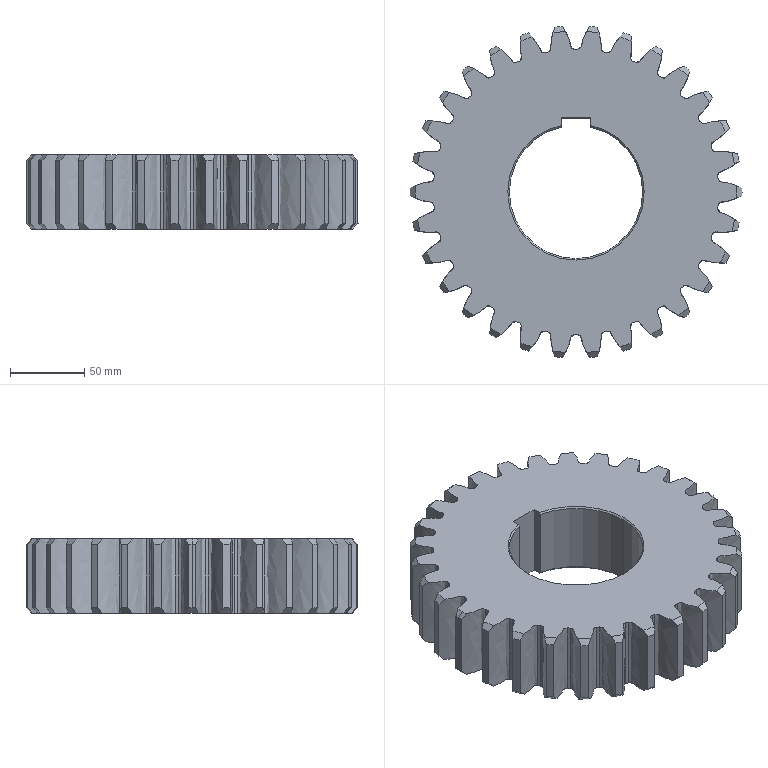Part | SolidWorks | features BaseBody 1 | 1 solid | 197 faces | box 224 x 223.253 x 50 mm | volume 1384242 mm3 | cone 68 | cylinder 64 | spline 60 | plane 5 | commonest cylinder face diameters 224 x31 192.5 x30 90 x3